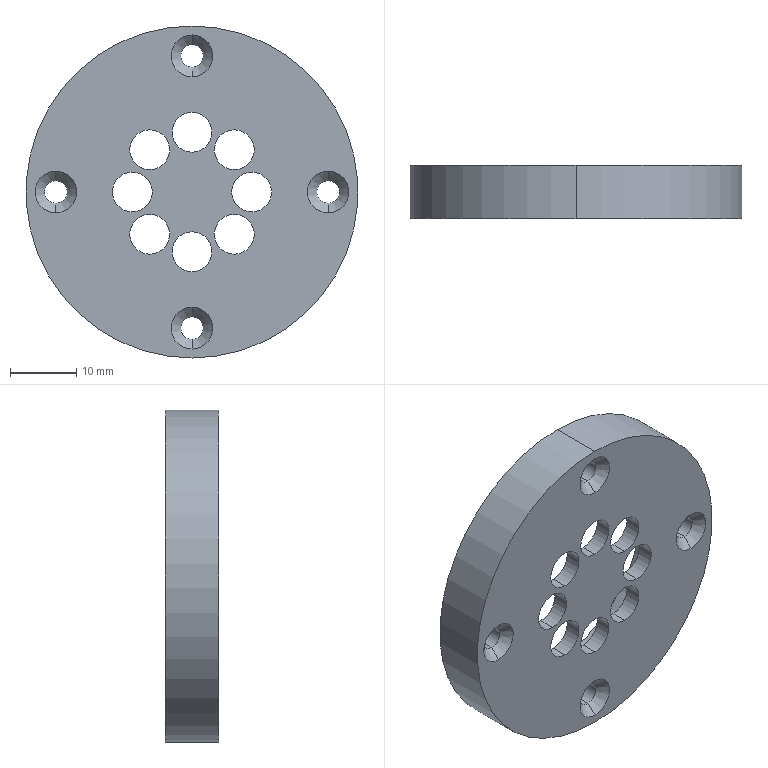Part | SolidWorks | features ICE 2, Extrusion 1, HoleWzd 1 | 1 solid | 39 faces | box 50 x 8 x 50 mm | volume 9503 mm3 | cylinder 28 | cone 8 | plane 3 | commonest cylinder face diameters 6 x16 3.4 x8 35 x2 50 x2
STEP:
#1=CARTESIAN_POINT('',(0.,1.45,-18.8));
#2=VERTEX_POINT('',#1);
#3=CARTESIAN_POINT('',(0.,1.45,-22.2));
#4=VERTEX_POINT('',#3);
#5=CARTESIAN_POINT('',(0.,1.45,-20.5));
#6=DIRECTION('',(0.,-1.,0.));
#7=DIRECTION('',(0.,0.,-1.));
#8=AXIS2_PLACEMENT_3D('',#5,#6,#7);
#9=CIRCLE('',#8,1.7);
#10=EDGE_CURVE('',#2,#4,#9,.T.);
#11=ORIENTED_EDGE('',*,*,#10,.F.);
#12=CARTESIAN_POINT('',(0.,0.,-17.35));
#13=VERTEX_POINT('',#12);
#14=CARTESIAN_POINT('',(0.,0.,-17.35));
#15=DIRECTION('',(0.,-0.7071,0.7071));
#16=VECTOR('',#15,1000.);
#17=LINE('',#14,#16);
#18=EDGE_CURVE('',#2,#13,#17,.T.);
#19=ORIENTED_EDGE('',*,*,#18,.T.);
#20=CARTESIAN_POINT('',(0.,0.,-23.65));
#21=VERTEX_POINT('',#20);
#22=CARTESIAN_POINT('',(0.,0.,-20.5));
#23=DIRECTION('',(0.,-1.,0.));
#24=DIRECTION('',(0.,0.,-1.));
#25=AXIS2_PLACEMENT_3D('',#22,#23,#24);
#26=CIRCLE('',#25,3.15);
#27=EDGE_CURVE('',#13,#21,#26,.T.);
#28=ORIENTED_EDGE('',*,*,#27,.T.);
#29=CARTESIAN_POINT('',(0.,0.,-23.65));
#30=DIRECTION('',(0.,-0.7071,-0.7071));
#31=VECTOR('',#30,1000.);
#32=LINE('',#29,#31);
#33=EDGE_CURVE('',#4,#21,#32,.T.);
#34=ORIENTED_EDGE('',*,*,#33,.F.);
#35=EDGE_LOOP('',(#11,#19,#28,#34));
#36=FACE_OUTER_BOUND('',#35,.T.);
#37=CARTESIAN_POINT('',(0.,0.,-20.5));
#38=DIRECTION('',(0.,-1.,0.));
#39=DIRECTION('',(0.,0.,-1.));
#40=AXIS2_PLACEMENT_3D('',#37,#38,#39);
#41=CONICAL_SURFACE('',#40,3.15,0.7854);
#42=ADVANCED_FACE('',(#36),#41,.F.);
#43=CARTESIAN_POINT('',(0.,8.,-18.8));
#44=VERTEX_POINT('',#43);
#45=CARTESIAN_POINT('',(0.,8.,-22.2));
#46=VERTEX_POINT('',#45);
#47=CARTESIAN_POINT('',(0.,8.,-20.5));
#48=DIRECTION('',(0.,-1.,0.));
#49=DIRECTION('',(0.,0.,-1.));
#50=AXIS2_PLACEMENT_3D('',#47,#48,#49);
#51=CIRCLE('',#50,1.7);
#52=EDGE_CURVE('',#44,#46,#51,.T.);
#53=ORIENTED_EDGE('',*,*,#52,.F.);
#54=CARTESIAN_POINT('',(0.,0.,-18.8));
#55=DIRECTION('',(0.,-1.,0.));
#56=VECTOR('',#55,1000.);
#57=LINE('',#54,#56);
#58=EDGE_CURVE('',#44,#2,#57,.T.);
#59=ORIENTED_EDGE('',*,*,#58,.T.);
#60=ORIENTED_EDGE('',*,*,#10,.T.);
#61=CARTESIAN_POINT('',(0.,0.,-22.2));
#62=DIRECTION('',(0.,-1.,0.));
#63=VECTOR('',#62,1000.);
#64=LINE('',#61,#63);
#65=EDGE_CURVE('',#46,#4,#64,.T.);
#66=ORIENTED_EDGE('',*,*,#65,.F.);
#67=EDGE_LOOP('',(#53,#59,#60,#66));
#68=FACE_OUTER_BOUND('',#67,.T.);
#69=CARTESIAN_POINT('',(0.,0.,-20.5));
#70=DIRECTION('',(0.,-1.,0.));
#71=DIRECTION('',(0.,0.,-1.));
#72=AXIS2_PLACEMENT_3D('',#69,#70,#71);
#73=CYLINDRICAL_SURFACE('',#72,1.7);
#74=ADVANCED_FACE('',(#68),#73,.F.);
#75=CARTESIAN_POINT('',(20.5,1.45,1.7));
#76=VERTEX_POINT('',#75);
#77=CARTESIAN_POINT('',(20.5,1.45,-1.7));
#78=VERTEX_POINT('',#77);
#79=CARTESIAN_POINT('',(20.5,1.45,0.));
#80=DIRECTION('',(0.,-1.,0.));
#81=DIRECTION('',(0.,0.,-1.));
#82=AXIS2_PLACEMENT_3D('',#79,#80,#81);
#83=CIRCLE('',#82,1.7);
#84=EDGE_CURVE('',#76,#78,#83,.T.);
#85=ORIENTED_EDGE('',*,*,#84,.F.);
#86=CARTESIAN_POINT('',(20.5,0.,3.15));
#87=VERTEX_POINT('',#86);
#88=CARTESIAN_POINT('',(20.5,0.,3.15));
#89=DIRECTION('',(0.,-0.7071,0.7071));
#90=VECTOR('',#89,1000.);
#91=LINE('',#88,#90);
#92=EDGE_CURVE('',#76,#87,#91,.T.);
#93=ORIENTED_EDGE('',*,*,#92,.T.);
#94=CARTESIAN_POINT('',(20.5,0.,-3.15));
#95=VERTEX_POINT('',#94);
#96=CARTESIAN_POINT('',(20.5,0.,0.));
#97=DIRECTION('',(0.,-1.,0.));
#98=DIRECTION('',(0.,0.,-1.));
#99=AXIS2_PLACEMENT_3D('',#96,#97,#98);
#100=CIRCLE('',#99,3.15);
#101=EDGE_CURVE('',#87,#95,#100,.T.);
#102=ORIENTED_EDGE('',*,*,#101,.T.);
#103=CARTESIAN_POINT('',(20.5,0.,-3.15));
#104=DIRECTION('',(0.,-0.7071,-0.7071));
#105=VECTOR('',#104,1000.);
#106=LINE('',#103,#105);
#107=EDGE_CURVE('',#78,#95,#106,.T.);
#108=ORIENTED_EDGE('',*,*,#107,.F.);
#109=EDGE_LOOP('',(#85,#93,#102,#108));
#110=FACE_OUTER_BOUND('',#109,.T.);
#111=CARTESIAN_POINT('',(20.5,0.,0.));
#112=DIRECTION('',(0.,-1.,0.));
#113=DIRECTION('',(0.,0.,-1.));
#114=AXIS2_PLACEMENT_3D('',#111,#112,#113);
#115=CONICAL_SURFACE('',#114,3.15,0.7854);
#116=ADVANCED_FACE('',(#110),#115,.F.);
#117=CARTESIAN_POINT('',(20.5,8.,1.7));
#118=VERTEX_POINT('',#117);
#119=CARTESIAN_POINT('',(20.5,8.,-1.7));
#120=VERTEX_POINT('',#119);
#121=CARTESIAN_POINT('',(20.5,8.,0.));
#122=DIRECTION('',(0.,-1.,0.));
#123=DIRECTION('',(0.,0.,-1.));
#124=AXIS2_PLACEMENT_3D('',#121,#122,#123);
#125=CIRCLE('',#124,1.7);
#126=EDGE_CURVE('',#118,#120,#125,.T.);
#127=ORIENTED_EDGE('',*,*,#126,.F.);
#128=CARTESIAN_POINT('',(20.5,0.,1.7));
#129=DIRECTION('',(0.,-1.,0.));
#130=VECTOR('',#129,1000.);
#131=LINE('',#128,#130);
#132=EDGE_CURVE('',#118,#76,#131,.T.);
#133=ORIENTED_EDGE('',*,*,#132,.T.);
#134=ORIENTED_EDGE('',*,*,#84,.T.);
#135=CARTESIAN_POINT('',(20.5,0.,-1.7));
#136=DIRECTION('',(0.,-1.,0.));
#137=VECTOR('',#136,1000.);
#138=LINE('',#135,#137);
#139=EDGE_CURVE('',#120,#78,#138,.T.);
#140=ORIENTED_EDGE('',*,*,#139,.F.);
#141=EDGE_LOOP('',(#127,#133,#134,#140));
#142=FACE_OUTER_BOUND('',#141,.T.);
#143=CARTESIAN_POINT('',(20.5,0.,0.));
#144=DIRECTION('',(0.,-1.,0.));
#145=DIRECTION('',(0.,0.,-1.));
#146=AXIS2_PLACEMENT_3D('',#143,#144,#145);
#147=CYLINDRICAL_SURFACE('',#146,1.7);
#148=ADVANCED_FACE('',(#142),#147,.F.);
#149=CARTESIAN_POINT('',(0.,1.45,22.2));
#150=VERTEX_POINT('',#149);
#151=CARTESIAN_POINT('',(0.,1.45,18.8));
#152=VERTEX_POINT('',#151);
#153=CARTESIAN_POINT('',(0.,1.45,20.5));
#154=DIRECTION('',(0.,-1.,0.));
#155=DIRECTION('',(0.,0.,-1.));
#156=AXIS2_PLACEMENT_3D('',#153,#154,#155);
#157=CIRCLE('',#156,1.7);
#158=EDGE_CURVE('',#150,#152,#157,.T.);
#159=ORIENTED_EDGE('',*,*,#158,.F.);
#160=CARTESIAN_POINT('',(0.,0.,23.65));
#161=VERTEX_POINT('',#160);
#162=CARTESIAN_POINT('',(0.,0.,23.65));
#163=DIRECTION('',(0.,-0.7071,0.7071));
#164=VECTOR('',#163,1000.);
#165=LINE('',#162,#164);
#166=EDGE_CURVE('',#150,#161,#165,.T.);
#167=ORIENTED_EDGE('',*,*,#166,.T.);
#168=CARTESIAN_POINT('',(0.,0.,17.35));
#169=VERTEX_POINT('',#168);
#170=CARTESIAN_POINT('',(0.,0.,20.5));
#171=DIRECTION('',(0.,-1.,0.));
#172=DIRECTION('',(0.,0.,-1.));
#173=AXIS2_PLACEMENT_3D('',#170,#171,#172);
#174=CIRCLE('',#173,3.15);
#175=EDGE_CURVE('',#161,#169,#174,.T.);
#176=ORIENTED_EDGE('',*,*,#175,.T.);
#177=CARTESIAN_POINT('',(0.,0.,17.35));
#178=DIRECTION('',(0.,-0.7071,-0.7071));
#179=VECTOR('',#178,1000.);
#180=LINE('',#177,#179);
#181=EDGE_CURVE('',#152,#169,#180,.T.);
#182=ORIENTED_EDGE('',*,*,#181,.F.);
#183=EDGE_LOOP('',(#159,#167,#176,#182));
#184=FACE_OUTER_BOUND('',#183,.T.);
#185=CARTESIAN_POINT('',(0.,0.,20.5));
#186=DIRECTION('',(0.,-1.,0.));
#187=DIRECTION('',(0.,0.,-1.));
#188=AXIS2_PLACEMENT_3D('',#185,#186,#187);
#189=CONICAL_SURFACE('',#188,3.15,0.7854);
#190=ADVANCED_FACE('',(#184),#189,.F.);
#191=CARTESIAN_POINT('',(0.,8.,22.2));
#192=VERTEX_POINT('',#191);
#193=CARTESIAN_POINT('',(0.,8.,18.8));
#194=VERTEX_POINT('',#193);
#195=CARTESIAN_POINT('',(0.,8.,20.5));
#196=DIRECTION('',(0.,-1.,0.));
#197=DIRECTION('',(0.,0.,-1.));
#198=AXIS2_PLACEMENT_3D('',#195,#196,#197);
#199=CIRCLE('',#198,1.7);
#200=EDGE_CURVE('',#192,#194,#199,.T.);
#201=ORIENTED_EDGE('',*,*,#200,.F.);
#202=CARTESIAN_POINT('',(0.,0.,22.2));
#203=DIRECTION('',(0.,-1.,0.));
#204=VECTOR('',#203,1000.);
#205=LINE('',#202,#204);
#206=EDGE_CURVE('',#192,#150,#205,.T.);
#207=ORIENTED_EDGE('',*,*,#206,.T.);
#208=ORIENTED_EDGE('',*,*,#158,.T.);
#209=CARTESIAN_POINT('',(0.,0.,18.8));
#210=DIRECTION('',(0.,-1.,0.));
#211=VECTOR('',#210,1000.);
#212=LINE('',#209,#211);
#213=EDGE_CURVE('',#194,#152,#212,.T.);
#214=ORIENTED_EDGE('',*,*,#213,.F.);
#215=EDGE_LOOP('',(#201,#207,#208,#214));
#216=FACE_OUTER_BOUND('',#215,.T.);
#217=CARTESIAN_POINT('',(0.,0.,20.5));
#218=DIRECTION('',(0.,-1.,0.));
#219=DIRECTION('',(0.,0.,-1.));
#220=AXIS2_PLACEMENT_3D('',#217,#218,#219);
#221=CYLINDRICAL_SURFACE('',#220,1.7);
#222=ADVANCED_FACE('',(#216),#221,.F.);
#223=CARTESIAN_POINT('',(-20.5,1.45,1.7));
#224=VERTEX_POINT('',#223);
#225=CARTESIAN_POINT('',(-20.5,1.45,-1.7));
#226=VERTEX_POINT('',#225);
#227=CARTESIAN_POINT('',(-20.5,1.45,0.));
#228=DIRECTION('',(0.,-1.,0.));
#229=DIRECTION('',(0.,0.,-1.));
#230=AXIS2_PLACEMENT_3D('',#227,#228,#229);
#231=CIRCLE('',#230,1.7);
#232=EDGE_CURVE('',#224,#226,#231,.T.);
#233=ORIENTED_EDGE('',*,*,#232,.F.);
#234=CARTESIAN_POINT('',(-20.5,0.,3.15));
#235=VERTEX_POINT('',#234);
#236=CARTESIAN_POINT('',(-20.5,0.,3.15));
#237=DIRECTION('',(0.,-0.7071,0.7071));
#238=VECTOR('',#237,1000.);
#239=LINE('',#236,#238);
#240=EDGE_CURVE('',#224,#235,#239,.T.);
#241=ORIENTED_EDGE('',*,*,#240,.T.);
#242=CARTESIAN_POINT('',(-20.5,0.,-3.15));
#243=VERTEX_POINT('',#242);
#244=CARTESIAN_POINT('',(-20.5,0.,0.));
#245=DIRECTION('',(0.,-1.,0.));
#246=DIRECTION('',(0.,0.,-1.));
#247=AXIS2_PLACEMENT_3D('',#244,#245,#246);
#248=CIRCLE('',#247,3.15);
#249=EDGE_CURVE('',#235,#243,#248,.T.);
#250=ORIENTED_EDGE('',*,*,#249,.T.);
#251=CARTESIAN_POINT('',(-20.5,0.,-3.15));
#252=DIRECTION('',(0.,-0.7071,-0.7071));
#253=VECTOR('',#252,1000.);
#254=LINE('',#251,#253);
#255=EDGE_CURVE('',#226,#243,#254,.T.);
#256=ORIENTED_EDGE('',*,*,#255,.F.);
#257=EDGE_LOOP('',(#233,#241,#250,#256));
#258=FACE_OUTER_BOUND('',#257,.T.);
#259=CARTESIAN_POINT('',(-20.5,0.,0.));
#260=DIRECTION('',(0.,-1.,0.));
#261=DIRECTION('',(0.,0.,-1.));
#262=AXIS2_PLACEMENT_3D('',#259,#260,#261);
#263=CONICAL_SURFACE('',#262,3.15,0.7854);
#264=ADVANCED_FACE('',(#258),#263,.F.);
#265=CARTESIAN_POINT('',(-20.5,8.,1.7));
#266=VERTEX_POINT('',#265);
#267=CARTESIAN_POINT('',(-20.5,8.,-1.7));
#268=VERTEX_POINT('',#267);
#269=CARTESIAN_POINT('',(-20.5,8.,0.));
#270=DIRECTION('',(0.,-1.,0.));
#271=DIRECTION('',(0.,0.,-1.));
#272=AXIS2_PLACEMENT_3D('',#269,#270,#271);
#273=CIRCLE('',#272,1.7);
#274=EDGE_CURVE('',#266,#268,#273,.T.);
#275=ORIENTED_EDGE('',*,*,#274,.F.);
#276=CARTESIAN_POINT('',(-20.5,0.,1.7));
#277=DIRECTION('',(0.,-1.,0.));
#278=VECTOR('',#277,1000.);
#279=LINE('',#276,#278);
#280=EDGE_CURVE('',#266,#224,#279,.T.);
#281=ORIENTED_EDGE('',*,*,#280,.T.);
#282=ORIENTED_EDGE('',*,*,#232,.T.);
#283=CARTESIAN_POINT('',(-20.5,0.,-1.7));
#284=DIRECTION('',(0.,-1.,0.));
#285=VECTOR('',#284,1000.);
#286=LINE('',#283,#285);
#287=EDGE_CURVE('',#268,#226,#286,.T.);
#288=ORIENTED_EDGE('',*,*,#287,.F.);
#289=EDGE_LOOP('',(#275,#281,#282,#288));
#290=FACE_OUTER_BOUND('',#289,.T.);
#291=CARTESIAN_POINT('',(-20.5,0.,0.));
#292=DIRECTION('',(0.,-1.,0.));
#293=DIRECTION('',(0.,0.,-1.));
#294=AXIS2_PLACEMENT_3D('',#291,#292,#293);
#295=CYLINDRICAL_SURFACE('',#294,1.7);
#296=ADVANCED_FACE('',(#290),#295,.F.);
#297=CARTESIAN_POINT('',(6.364,2.5,-9.364));
#298=VERTEX_POINT('',#297);
#299=CARTESIAN_POINT('',(6.364,2.5,-3.364));
#300=VERTEX_POINT('',#299);
#301=CARTESIAN_POINT('',(6.364,2.5,-6.364));
#302=DIRECTION('',(0.,1.,0.));
#303=DIRECTION('',(0.,0.,1.));
#304=AXIS2_PLACEMENT_3D('',#301,#302,#303);
#305=CIRCLE('',#304,3.);
#306=EDGE_CURVE('',#298,#300,#305,.T.);
#307=ORIENTED_EDGE('',*,*,#306,.T.);
#308=CARTESIAN_POINT('',(6.364,0.,-3.364));
#309=VERTEX_POINT('',#308);
#310=CARTESIAN_POINT('',(6.364,4.,-3.364));
#311=DIRECTION('',(0.,-1.,0.));
#312=VECTOR('',#311,1000.);
#313=LINE('',#310,#312);
#314=EDGE_CURVE('',#300,#309,#313,.T.);
#315=ORIENTED_EDGE('',*,*,#314,.T.);
#316=CARTESIAN_POINT('',(6.364,0.,-9.364));
#317=VERTEX_POINT('',#316);
#318=CARTESIAN_POINT('',(6.364,0.,-6.364));
#319=DIRECTION('',(0.,-1.,0.));
#320=DIRECTION('',(0.,0.,-1.));
#321=AXIS2_PLACEMENT_3D('',#318,#319,#320);
#322=CIRCLE('',#321,3.);
#323=EDGE_CURVE('',#309,#317,#322,.T.);
#324=ORIENTED_EDGE('',*,*,#323,.T.);
#325=CARTESIAN_POINT('',(6.364,4.,-9.364));
#326=DIRECTION('',(0.,-1.,0.));
#327=VECTOR('',#326,1000.);
#328=LINE('',#325,#327);
#329=EDGE_CURVE('',#298,#317,#328,.T.);
#330=ORIENTED_EDGE('',*,*,#329,.F.);
#331=EDGE_LOOP('',(#307,#315,#324,#330));
#332=FACE_OUTER_BOUND('',#331,.T.);
#333=CARTESIAN_POINT('',(6.364,4.,-6.364));
#334=DIRECTION('',(0.,-1.,0.));
#335=DIRECTION('',(0.,0.,-1.));
#336=AXIS2_PLACEMENT_3D('',#333,#334,#335);
#337=CYLINDRICAL_SURFACE('',#336,3.);
#338=ADVANCED_FACE('',(#332),#337,.F.);
#339=CARTESIAN_POINT('',(9.,2.5,-3.));
#340=VERTEX_POINT('',#339);
#341=CARTESIAN_POINT('',(9.,2.5,3.));
#342=VERTEX_POINT('',#341);
#343=CARTESIAN_POINT('',(9.,2.5,0.));
#344=DIRECTION('',(0.,1.,0.));
#345=DIRECTION('',(0.,0.,1.));
#346=AXIS2_PLACEMENT_3D('',#343,#344,#345);
#347=CIRCLE('',#346,3.);
#348=EDGE_CURVE('',#340,#342,#347,.T.);
#349=ORIENTED_EDGE('',*,*,#348,.T.);
#350=CARTESIAN_POINT('',(9.,0.,3.));
#351=VERTEX_POINT('',#350);
#352=CARTESIAN_POINT('',(9.,4.,3.));
#353=DIRECTION('',(0.,-1.,0.));
#354=VECTOR('',#353,1000.);
#355=LINE('',#352,#354);
#356=EDGE_CURVE('',#342,#351,#355,.T.);
#357=ORIENTED_EDGE('',*,*,#356,.T.);
#358=CARTESIAN_POINT('',(9.,0.,-3.));
#359=VERTEX_POINT('',#358);
#360=CARTESIAN_POINT('',(9.,0.,0.));
#361=DIRECTION('',(0.,-1.,0.));
#362=DIRECTION('',(0.,0.,-1.));
#363=AXIS2_PLACEMENT_3D('',#360,#361,#362);
#364=CIRCLE('',#363,3.);
#365=EDGE_CURVE('',#351,#359,#364,.T.);
#366=ORIENTED_EDGE('',*,*,#365,.T.);
#367=CARTESIAN_POINT('',(9.,4.,-3.));
#368=DIRECTION('',(0.,-1.,0.));
#369=VECTOR('',#368,1000.);
#370=LINE('',#367,#369);
#371=EDGE_CURVE('',#340,#359,#370,.T.);
#372=ORIENTED_EDGE('',*,*,#371,.F.);
#373=EDGE_LOOP('',(#349,#357,#366,#372));
#374=FACE_OUTER_BOUND('',#373,.T.);
#375=CARTESIAN_POINT('',(9.,4.,0.));
#376=DIRECTION('',(0.,-1.,0.));
#377=DIRECTION('',(0.,0.,-1.));
#378=AXIS2_PLACEMENT_3D('',#375,#376,#377);
#379=CYLINDRICAL_SURFACE('',#378,3.);
#380=ADVANCED_FACE('',(#374),#379,.F.);
#381=CARTESIAN_POINT('',(6.364,2.5,3.364));
#382=VERTEX_POINT('',#381);
#383=CARTESIAN_POINT('',(6.364,2.5,9.364));
#384=VERTEX_POINT('',#383);
#385=CARTESIAN_POINT('',(6.364,2.5,6.364));
#386=DIRECTION('',(0.,1.,0.));
#387=DIRECTION('',(0.,0.,1.));
#388=AXIS2_PLACEMENT_3D('',#385,#386,#387);
#389=CIRCLE('',#388,3.);
#390=EDGE_CURVE('',#382,#384,#389,.T.);
#391=ORIENTED_EDGE('',*,*,#390,.T.);
#392=CARTESIAN_POINT('',(6.364,0.,9.364));
#393=VERTEX_POINT('',#392);
#394=CARTESIAN_POINT('',(6.364,4.,9.364));
#395=DIRECTION('',(0.,-1.,0.));
#396=VECTOR('',#395,1000.);
#397=LINE('',#394,#396);
#398=EDGE_CURVE('',#384,#393,#397,.T.);
#399=ORIENTED_EDGE('',*,*,#398,.T.);
#400=CARTESIAN_POINT('',(6.364,0.,3.364));
#401=VERTEX_POINT('',#400);
#402=CARTESIAN_POINT('',(6.364,0.,6.364));
#403=DIRECTION('',(0.,-1.,0.));
#404=DIRECTION('',(0.,0.,-1.));
#405=AXIS2_PLACEMENT_3D('',#402,#403,#404);
#406=CIRCLE('',#405,3.);
#407=EDGE_CURVE('',#393,#401,#406,.T.);
#408=ORIENTED_EDGE('',*,*,#407,.T.);
#409=CARTESIAN_POINT('',(6.364,4.,3.364));
#410=DIRECTION('',(0.,-1.,0.));
#411=VECTOR('',#410,1000.);
#412=LINE('',#409,#411);
#413=EDGE_CURVE('',#382,#401,#412,.T.);
#414=ORIENTED_EDGE('',*,*,#413,.F.);
#415=EDGE_LOOP('',(#391,#399,#408,#414));
#416=FACE_OUTER_BOUND('',#415,.T.);
#417=CARTESIAN_POINT('',(6.364,4.,6.364));
#418=DIRECTION('',(0.,-1.,0.));
#419=DIRECTION('',(0.,0.,-1.));
#420=AXIS2_PLACEMENT_3D('',#417,#418,#419);
#421=CYLINDRICAL_SURFACE('',#420,3.);
#422=ADVANCED_FACE('',(#416),#421,.F.);
#423=CARTESIAN_POINT('',(0.,2.5,6.));
#424=VERTEX_POINT('',#423);
#425=CARTESIAN_POINT('',(0.,2.5,12.));
#426=VERTEX_POINT('',#425);
#427=CARTESIAN_POINT('',(0.,2.5,9.));
#428=DIRECTION('',(0.,1.,0.));
#429=DIRECTION('',(0.,0.,1.));
#430=AXIS2_PLACEMENT_3D('',#427,#428,#429);
#431=CIRCLE('',#430,3.);
#432=EDGE_CURVE('',#424,#426,#431,.T.);
#433=ORIENTED_EDGE('',*,*,#432,.T.);
#434=CARTESIAN_POINT('',(0.,0.,12.));
#435=VERTEX_POINT('',#434);
#436=CARTESIAN_POINT('',(0.,4.,12.));
#437=DIRECTION('',(0.,-1.,0.));
#438=VECTOR('',#437,1000.);
#439=LINE('',#436,#438);
#440=EDGE_CURVE('',#426,#435,#439,.T.);
#441=ORIENTED_EDGE('',*,*,#440,.T.);
#442=CARTESIAN_POINT('',(0.,0.,6.));
#443=VERTEX_POINT('',#442);
#444=CARTESIAN_POINT('',(0.,0.,9.));
#445=DIRECTION('',(0.,-1.,0.));
#446=DIRECTION('',(0.,0.,-1.));
#447=AXIS2_PLACEMENT_3D('',#444,#445,#446);
#448=CIRCLE('',#447,3.);
#449=EDGE_CURVE('',#435,#443,#448,.T.);
#450=ORIENTED_EDGE('',*,*,#449,.T.);
#451=CARTESIAN_POINT('',(0.,4.,6.));
#452=DIRECTION('',(0.,-1.,0.));
#453=VECTOR('',#452,1000.);
#454=LINE('',#451,#453);
#455=EDGE_CURVE('',#424,#443,#454,.T.);
#456=ORIENTED_EDGE('',*,*,#455,.F.);
#457=EDGE_LOOP('',(#433,#441,#450,#456));
#458=FACE_OUTER_BOUND('',#457,.T.);
#459=CARTESIAN_POINT('',(0.,4.,9.));
#460=DIRECTION('',(0.,-1.,0.));
#461=DIRECTION('',(0.,0.,-1.));
#462=AXIS2_PLACEMENT_3D('',#459,#460,#461);
#463=CYLINDRICAL_SURFACE('',#462,3.);
#464=ADVANCED_FACE('',(#458),#463,.F.);
#465=CARTESIAN_POINT('',(-6.364,2.5,3.364));
#466=VERTEX_POINT('',#465);
#467=CARTESIAN_POINT('',(-6.364,2.5,9.364));
#468=VERTEX_POINT('',#467);
#469=CARTESIAN_POINT('',(-6.364,2.5,6.364));
#470=DIRECTION('',(0.,1.,0.));
#471=DIRECTION('',(0.,0.,1.));
#472=AXIS2_PLACEMENT_3D('',#469,#470,#471);
#473=CIRCLE('',#472,3.);
#474=EDGE_CURVE('',#466,#468,#473,.T.);
#475=ORIENTED_EDGE('',*,*,#474,.T.);
#476=CARTESIAN_POINT('',(-6.364,0.,9.364));
#477=VERTEX_POINT('',#476);
#478=CARTESIAN_POINT('',(-6.364,4.,9.364));
#479=DIRECTION('',(0.,-1.,0.));
#480=VECTOR('',#479,1000.);
#481=LINE('',#478,#480);
#482=EDGE_CURVE('',#468,#477,#481,.T.);
#483=ORIENTED_EDGE('',*,*,#482,.T.);
#484=CARTESIAN_POINT('',(-6.364,0.,3.364));
#485=VERTEX_POINT('',#484);
#486=CARTESIAN_POINT('',(-6.364,0.,6.364));
#487=DIRECTION('',(0.,-1.,0.));
#488=DIRECTION('',(0.,0.,-1.));
#489=AXIS2_PLACEMENT_3D('',#486,#487,#488);
#490=CIRCLE('',#489,3.);
#491=EDGE_CURVE('',#477,#485,#490,.T.);
#492=ORIENTED_EDGE('',*,*,#491,.T.);
#493=CARTESIAN_POINT('',(-6.364,4.,3.364));
#494=DIRECTION('',(0.,-1.,0.));
#495=VECTOR('',#494,1000.);
#496=LINE('',#493,#495);
#497=EDGE_CURVE('',#466,#485,#496,.T.);
#498=ORIENTED_EDGE('',*,*,#497,.F.);
#499=EDGE_LOOP('',(#475,#483,#492,#498));
#500=FACE_OUTER_BOUND('',#499,.T.);
#501=CARTESIAN_POINT('',(-6.364,4.,6.364));
#502=DIRECTION('',(0.,-1.,0.));
#503=DIRECTION('',(0.,0.,-1.));
#504=AXIS2_PLACEMENT_3D('',#501,#502,#503);
#505=CYLINDRICAL_SURFACE('',#504,3.);
#506=ADVANCED_FACE('',(#500),#505,.F.);
#507=CARTESIAN_POINT('',(-9.,2.5,-3.));
#508=VERTEX_POINT('',#507);
#509=CARTESIAN_POINT('',(-9.,2.5,3.));
#510=VERTEX_POINT('',#509);
#511=CARTESIAN_POINT('',(-9.,2.5,0.));
#512=DIRECTION('',(0.,1.,0.));
#513=DIRECTION('',(0.,0.,1.));
#514=AXIS2_PLACEMENT_3D('',#511,#512,#513);
#515=CIRCLE('',#514,3.);
#516=EDGE_CURVE('',#508,#510,#515,.T.);
#517=ORIENTED_EDGE('',*,*,#516,.T.);
#518=CARTESIAN_POINT('',(-9.,0.,3.));
#519=VERTEX_POINT('',#518);
#520=CARTESIAN_POINT('',(-9.,4.,3.));
#521=DIRECTION('',(0.,-1.,0.));
#522=VECTOR('',#521,1000.);
#523=LINE('',#520,#522);
#524=EDGE_CURVE('',#510,#519,#523,.T.);
#525=ORIENTED_EDGE('',*,*,#524,.T.);
#526=CARTESIAN_POINT('',(-9.,0.,-3.));
#527=VERTEX_POINT('',#526);
#528=CARTESIAN_POINT('',(-9.,0.,0.));
#529=DIRECTION('',(0.,-1.,0.));
#530=DIRECTION('',(0.,0.,-1.));
#531=AXIS2_PLACEMENT_3D('',#528,#529,#530);
#532=CIRCLE('',#531,3.);
#533=EDGE_CURVE('',#519,#527,#532,.T.);
#534=ORIENTED_EDGE('',*,*,#533,.T.);
#535=CARTESIAN_POINT('',(-9.,4.,-3.));
#536=DIRECTION('',(0.,-1.,0.));
#537=VECTOR('',#536,1000.);
#538=LINE('',#535,#537);
#539=EDGE_CURVE('',#508,#527,#538,.T.);
#540=ORIENTED_EDGE('',*,*,#539,.F.);
#541=EDGE_LOOP('',(#517,#525,#534,#540));
#542=FACE_OUTER_BOUND('',#541,.T.);
#543=CARTESIAN_POINT('',(-9.,4.,0.));
#544=DIRECTION('',(0.,-1.,0.));
#545=DIRECTION('',(0.,0.,-1.));
#546=AXIS2_PLACEMENT_3D('',#543,#544,#545);
#547=CYLINDRICAL_SURFACE('',#546,3.);
#548=ADVANCED_FACE('',(#542),#547,.F.);
#549=CARTESIAN_POINT('',(-6.364,2.5,-9.364));
#550=VERTEX_POINT('',#549);
#551=CARTESIAN_POINT('',(-6.364,2.5,-3.364));
#552=VERTEX_POINT('',#551);
#553=CARTESIAN_POINT('',(-6.364,2.5,-6.364));
#554=DIRECTION('',(0.,1.,0.));
#555=DIRECTION('',(0.,0.,1.));
#556=AXIS2_PLACEMENT_3D('',#553,#554,#555);
#557=CIRCLE('',#556,3.);
#558=EDGE_CURVE('',#550,#552,#557,.T.);
#559=ORIENTED_EDGE('',*,*,#558,.T.);
#560=CARTESIAN_POINT('',(-6.364,0.,-3.364));
#561=VERTEX_POINT('',#560);
#562=CARTESIAN_POINT('',(-6.364,4.,-3.364));
#563=DIRECTION('',(0.,-1.,0.));
#564=VECTOR('',#563,1000.);
#565=LINE('',#562,#564);
#566=EDGE_CURVE('',#552,#561,#565,.T.);
#567=ORIENTED_EDGE('',*,*,#566,.T.);
#568=CARTESIAN_POINT('',(-6.364,0.,-9.364));
#569=VERTEX_POINT('',#568);
#570=CARTESIAN_POINT('',(-6.364,0.,-6.364));
#571=DIRECTION('',(0.,-1.,0.));
#572=DIRECTION('',(0.,0.,-1.));
#573=AXIS2_PLACEMENT_3D('',#570,#571,#572);
#574=CIRCLE('',#573,3.);
#575=EDGE_CURVE('',#561,#569,#574,.T.);
#576=ORIENTED_EDGE('',*,*,#575,.T.);
#577=CARTESIAN_POINT('',(-6.364,4.,-9.364));
#578=DIRECTION('',(0.,-1.,0.));
#579=VECTOR('',#578,1000.);
#580=LINE('',#577,#579);
#581=EDGE_CURVE('',#550,#569,#580,.T.);
#582=ORIENTED_EDGE('',*,*,#581,.F.);
#583=EDGE_LOOP('',(#559,#567,#576,#582));
#584=FACE_OUTER_BOUND('',#583,.T.);
#585=CARTESIAN_POINT('',(-6.364,4.,-6.364));
#586=DIRECTION('',(0.,-1.,0.));
#587=DIRECTION('',(0.,0.,-1.));
#588=AXIS2_PLACEMENT_3D('',#585,#586,#587);
#589=CYLINDRICAL_SURFACE('',#588,3.);
#590=ADVANCED_FACE('',(#584),#589,.F.);
#591=CARTESIAN_POINT('',(0.,2.5,-12.));
#592=VERTEX_POINT('',#591);
#593=CARTESIAN_POINT('',(0.,2.5,-6.));
#594=VERTEX_POINT('',#593);
#595=CARTESIAN_POINT('',(0.,2.5,-9.));
#596=DIRECTION('',(0.,1.,0.));
#597=DIRECTION('',(0.,0.,1.));
#598=AXIS2_PLACEMENT_3D('',#595,#596,#597);
#599=CIRCLE('',#598,3.);
#600=EDGE_CURVE('',#592,#594,#599,.T.);
#601=ORIENTED_EDGE('',*,*,#600,.T.);
#602=CARTESIAN_POINT('',(0.,0.,-6.));
#603=VERTEX_POINT('',#602);
#604=CARTESIAN_POINT('',(0.,4.,-6.));
#605=DIRECTION('',(0.,-1.,0.));
#606=VECTOR('',#605,1000.);
#607=LINE('',#604,#606);
#608=EDGE_CURVE('',#594,#603,#607,.T.);
#609=ORIENTED_EDGE('',*,*,#608,.T.);
#610=CARTESIAN_POINT('',(0.,0.,-12.));
#611=VERTEX_POINT('',#610);
#612=CARTESIAN_POINT('',(0.,0.,-9.));
#613=DIRECTION('',(0.,-1.,0.));
#614=DIRECTION('',(0.,0.,-1.));
#615=AXIS2_PLACEMENT_3D('',#612,#613,#614);
#616=CIRCLE('',#615,3.);
#617=EDGE_CURVE('',#603,#611,#616,.T.);
#618=ORIENTED_EDGE('',*,*,#617,.T.);
#619=CARTESIAN_POINT('',(0.,4.,-12.));
#620=DIRECTION('',(0.,-1.,0.));
#621=VECTOR('',#620,1000.);
#622=LINE('',#619,#621);
#623=EDGE_CURVE('',#592,#611,#622,.T.);
#624=ORIENTED_EDGE('',*,*,#623,.F.);
#625=EDGE_LOOP('',(#601,#609,#618,#624));
#626=FACE_OUTER_BOUND('',#625,.T.);
#627=CARTESIAN_POINT('',(0.,4.,-9.));
#628=DIRECTION('',(0.,-1.,0.));
#629=DIRECTION('',(0.,0.,-1.));
#630=AXIS2_PLACEMENT_3D('',#627,#628,#629);
#631=CYLINDRICAL_SURFACE('',#630,3.);
#632=ADVANCED_FACE('',(#626),#631,.F.);
#633=CARTESIAN_POINT('',(0.,2.5,-17.5));
#634=VERTEX_POINT('',#633);
#635=CARTESIAN_POINT('',(0.,2.5,17.5));
#636=VERTEX_POINT('',#635);
#637=CARTESIAN_POINT('',(0.,2.5,0.));
#638=DIRECTION('',(0.,1.,0.));
#639=DIRECTION('',(0.,0.,1.));
#640=AXIS2_PLACEMENT_3D('',#637,#638,#639);
#641=CIRCLE('',#640,17.5);
#642=EDGE_CURVE('',#634,#636,#641,.T.);
#643=ORIENTED_EDGE('',*,*,#642,.F.);
#644=CARTESIAN_POINT('',(0.,8.,-17.5));
#645=VERTEX_POINT('',#644);
#646=CARTESIAN_POINT('',(0.,2.5,-17.5));
#647=DIRECTION('',(0.,1.,0.));
#648=VECTOR('',#647,1000.);
#649=LINE('',#646,#648);
#650=EDGE_CURVE('',#634,#645,#649,.T.);
#651=ORIENTED_EDGE('',*,*,#650,.T.);
#652=CARTESIAN_POINT('',(0.,8.,17.5));
#653=VERTEX_POINT('',#652);
#654=CARTESIAN_POINT('',(0.,8.,0.));
#655=DIRECTION('',(0.,1.,0.));
#656=DIRECTION('',(0.,0.,1.));
#657=AXIS2_PLACEMENT_3D('',#654,#655,#656);
#658=CIRCLE('',#657,17.5);
#659=EDGE_CURVE('',#645,#653,#658,.T.);
#660=ORIENTED_EDGE('',*,*,#659,.T.);
#661=CARTESIAN_POINT('',(0.,2.5,17.5));
#662=DIRECTION('',(0.,1.,0.));
#663=VECTOR('',#662,1000.);
#664=LINE('',#661,#663);
#665=EDGE_CURVE('',#636,#653,#664,.T.);
#666=ORIENTED_EDGE('',*,*,#665,.F.);
#667=EDGE_LOOP('',(#643,#651,#660,#666));
#668=FACE_OUTER_BOUND('',#667,.T.);
#669=CARTESIAN_POINT('',(0.,2.5,0.));
#670=DIRECTION('',(0.,1.,0.));
#671=DIRECTION('',(0.,0.,1.));
#672=AXIS2_PLACEMENT_3D('',#669,#670,#671);
#673=CYLINDRICAL_SURFACE('',#672,17.5);
#674=ADVANCED_FACE('',(#668),#673,.F.);
#675=CARTESIAN_POINT('',(0.,8.,25.));
#676=VERTEX_POINT('',#675);
#677=CARTESIAN_POINT('',(0.,8.,-25.));
#678=VERTEX_POINT('',#677);
#679=CARTESIAN_POINT('',(0.,8.,0.));
#680=DIRECTION('',(0.,1.,0.));
#681=DIRECTION('',(0.,0.,1.));
#682=AXIS2_PLACEMENT_3D('',#679,#680,#681);
#683=CIRCLE('',#682,25.);
#684=EDGE_CURVE('',#676,#678,#683,.T.);
#685=ORIENTED_EDGE('',*,*,#684,.F.);
#686=CARTESIAN_POINT('',(0.,0.,25.));
#687=VERTEX_POINT('',#686);
#688=CARTESIAN_POINT('',(0.,8.,25.));
#689=DIRECTION('',(0.,-1.,0.));
#690=VECTOR('',#689,1000.);
#691=LINE('',#688,#690);
#692=EDGE_CURVE('',#676,#687,#691,.T.);
#693=ORIENTED_EDGE('',*,*,#692,.T.);
#694=CARTESIAN_POINT('',(0.,0.,-25.));
#695=VERTEX_POINT('',#694);
#696=CARTESIAN_POINT('',(0.,0.,0.));
#697=DIRECTION('',(0.,1.,0.));
#698=DIRECTION('',(0.,0.,1.));
#699=AXIS2_PLACEMENT_3D('',#696,#697,#698);
#700=CIRCLE('',#699,25.);
#701=EDGE_CURVE('',#687,#695,#700,.T.);
#702=ORIENTED_EDGE('',*,*,#701,.T.);
#703=CARTESIAN_POINT('',(0.,8.,-25.));
#704=DIRECTION('',(0.,-1.,0.));
#705=VECTOR('',#704,1000.);
#706=LINE('',#703,#705);
#707=EDGE_CURVE('',#678,#695,#706,.T.);
#708=ORIENTED_EDGE('',*,*,#707,.F.);
#709=EDGE_LOOP('',(#685,#693,#702,#708));
#710=FACE_OUTER_BOUND('',#709,.T.);
#711=CARTESIAN_POINT('',(0.,8.,0.));
#712=DIRECTION('',(0.,-1.,0.));
#713=DIRECTION('',(0.,0.,-1.));
#714=AXIS2_PLACEMENT_3D('',#711,#712,#713);
#715=CYLINDRICAL_SURFACE('',#714,25.);
#716=ADVANCED_FACE('',(#710),#715,.T.);
#717=CARTESIAN_POINT('',(20.5,8.,0.));
#718=DIRECTION('',(0.,-1.,0.));
#719=DIRECTION('',(0.,0.,-1.));
#720=AXIS2_PLACEMENT_3D('',#717,#718,#719);
#721=CIRCLE('',#720,1.7);
#722=EDGE_CURVE('',#120,#118,#721,.T.);
#723=ORIENTED_EDGE('',*,*,#722,.T.);
#724=ORIENTED_EDGE('',*,*,#126,.T.);
#725=EDGE_LOOP('',(#723,#724));
#726=FACE_BOUND('',#725,.T.);
#727=CARTESIAN_POINT('',(-20.5,8.,0.));
#728=DIRECTION('',(0.,-1.,0.));
#729=DIRECTION('',(0.,0.,-1.));
#730=AXIS2_PLACEMENT_3D('',#727,#728,#729);
#731=CIRCLE('',#730,1.7);
#732=EDGE_CURVE('',#268,#266,#731,.T.);
#733=ORIENTED_EDGE('',*,*,#732,.T.);
#734=ORIENTED_EDGE('',*,*,#274,.T.);
#735=EDGE_LOOP('',(#733,#734));
#736=FACE_BOUND('',#735,.T.);
#737=CARTESIAN_POINT('',(0.,8.,0.));
#738=DIRECTION('',(0.,1.,0.));
#739=DIRECTION('',(0.,0.,1.));
#740=AXIS2_PLACEMENT_3D('',#737,#738,#739);
#741=CIRCLE('',#740,17.5);
#742=EDGE_CURVE('',#653,#645,#741,.T.);
#743=ORIENTED_EDGE('',*,*,#742,.F.);
#744=ORIENTED_EDGE('',*,*,#659,.F.);
#745=EDGE_LOOP('',(#743,#744));
#746=FACE_BOUND('',#745,.T.);
#747=CARTESIAN_POINT('',(0.,8.,0.));
#748=DIRECTION('',(0.,1.,0.));
#749=DIRECTION('',(0.,0.,1.));
#750=AXIS2_PLACEMENT_3D('',#747,#748,#749);
#751=CIRCLE('',#750,25.);
#752=EDGE_CURVE('',#678,#676,#751,.T.);
#753=ORIENTED_EDGE('',*,*,#752,.T.);
#754=ORIENTED_EDGE('',*,*,#684,.T.);
#755=EDGE_LOOP('',(#753,#754));
#756=FACE_OUTER_BOUND('',#755,.T.);
#757=CARTESIAN_POINT('',(0.,8.,20.5));
#758=DIRECTION('',(0.,-1.,0.));
#759=DIRECTION('',(0.,0.,-1.));
#760=AXIS2_PLACEMENT_3D('',#757,#758,#759);
#761=CIRCLE('',#760,1.7);
#762=EDGE_CURVE('',#194,#192,#761,.T.);
#763=ORIENTED_EDGE('',*,*,#762,.T.);
#764=ORIENTED_EDGE('',*,*,#200,.T.);
#765=EDGE_LOOP('',(#763,#764));
#766=FACE_BOUND('',#765,.T.);
#767=CARTESIAN_POINT('',(0.,8.,-20.5));
#768=DIRECTION('',(0.,-1.,0.));
#769=DIRECTION('',(0.,0.,-1.));
#770=AXIS2_PLACEMENT_3D('',#767,#768,#769);
#771=CIRCLE('',#770,1.7);
#772=EDGE_CURVE('',#46,#44,#771,.T.);
#773=ORIENTED_EDGE('',*,*,#772,.T.);
#774=ORIENTED_EDGE('',*,*,#52,.T.);
#775=EDGE_LOOP('',(#773,#774));
#776=FACE_BOUND('',#775,.T.);
#777=CARTESIAN_POINT('',(0.,8.,0.));
#778=DIRECTION('',(0.,1.,0.));
#779=DIRECTION('',(0.,0.,1.));
#780=AXIS2_PLACEMENT_3D('',#777,#778,#779);
#781=PLANE('',#780);
#782=ADVANCED_FACE('',(#726,#736,#746,#756,#766,#776),#781,.T.);
#783=CARTESIAN_POINT('',(20.5,0.,0.));
#784=DIRECTION('',(0.,-1.,0.));
#785=DIRECTION('',(0.,0.,-1.));
#786=AXIS2_PLACEMENT_3D('',#783,#784,#785);
#787=CIRCLE('',#786,3.15);
#788=EDGE_CURVE('',#95,#87,#787,.T.);
#789=ORIENTED_EDGE('',*,*,#788,.F.);
#790=ORIENTED_EDGE('',*,*,#101,.F.);
#791=EDGE_LOOP('',(#789,#790));
#792=FACE_BOUND('',#791,.T.);
#793=CARTESIAN_POINT('',(-20.5,0.,0.));
#794=DIRECTION('',(0.,-1.,0.));
#795=DIRECTION('',(0.,0.,-1.));
#796=AXIS2_PLACEMENT_3D('',#793,#794,#795);
#797=CIRCLE('',#796,3.15);
#798=EDGE_CURVE('',#243,#235,#797,.T.);
#799=ORIENTED_EDGE('',*,*,#798,.F.);
#800=ORIENTED_EDGE('',*,*,#249,.F.);
#801=EDGE_LOOP('',(#799,#800));
#802=FACE_BOUND('',#801,.T.);
#803=CARTESIAN_POINT('',(6.364,0.,-6.364));
#804=DIRECTION('',(0.,-1.,0.));
#805=DIRECTION('',(0.,0.,-1.));
#806=AXIS2_PLACEMENT_3D('',#803,#804,#805);
#807=CIRCLE('',#806,3.);
#808=EDGE_CURVE('',#317,#309,#807,.T.);
#809=ORIENTED_EDGE('',*,*,#808,.F.);
#810=ORIENTED_EDGE('',*,*,#323,.F.);
#811=EDGE_LOOP('',(#809,#810));
#812=FACE_BOUND('',#811,.T.);
#813=CARTESIAN_POINT('',(9.,0.,0.));
#814=DIRECTION('',(0.,-1.,0.));
#815=DIRECTION('',(0.,0.,-1.));
#816=AXIS2_PLACEMENT_3D('',#813,#814,#815);
#817=CIRCLE('',#816,3.);
#818=EDGE_CURVE('',#359,#351,#817,.T.);
#819=ORIENTED_EDGE('',*,*,#818,.F.);
#820=ORIENTED_EDGE('',*,*,#365,.F.);
#821=EDGE_LOOP('',(#819,#820));
#822=FACE_BOUND('',#821,.T.);
#823=CARTESIAN_POINT('',(6.364,0.,6.364));
#824=DIRECTION('',(0.,-1.,0.));
#825=DIRECTION('',(0.,0.,-1.));
#826=AXIS2_PLACEMENT_3D('',#823,#824,#825);
#827=CIRCLE('',#826,3.);
#828=EDGE_CURVE('',#401,#393,#827,.T.);
#829=ORIENTED_EDGE('',*,*,#828,.F.);
#830=ORIENTED_EDGE('',*,*,#407,.F.);
#831=EDGE_LOOP('',(#829,#830));
#832=FACE_BOUND('',#831,.T.);
#833=CARTESIAN_POINT('',(0.,0.,9.));
#834=DIRECTION('',(0.,-1.,0.));
#835=DIRECTION('',(0.,0.,-1.));
#836=AXIS2_PLACEMENT_3D('',#833,#834,#835);
#837=CIRCLE('',#836,3.);
#838=EDGE_CURVE('',#443,#435,#837,.T.);
#839=ORIENTED_EDGE('',*,*,#838,.F.);
#840=ORIENTED_EDGE('',*,*,#449,.F.);
#841=EDGE_LOOP('',(#839,#840));
#842=FACE_BOUND('',#841,.T.);
#843=CARTESIAN_POINT('',(-6.364,0.,6.364));
#844=DIRECTION('',(0.,-1.,0.));
#845=DIRECTION('',(0.,0.,-1.));
#846=AXIS2_PLACEMENT_3D('',#843,#844,#845);
#847=CIRCLE('',#846,3.);
#848=EDGE_CURVE('',#485,#477,#847,.T.);
#849=ORIENTED_EDGE('',*,*,#848,.F.);
#850=ORIENTED_EDGE('',*,*,#491,.F.);
#851=EDGE_LOOP('',(#849,#850));
#852=FACE_BOUND('',#851,.T.);
#853=CARTESIAN_POINT('',(-9.,0.,0.));
#854=DIRECTION('',(0.,-1.,0.));
#855=DIRECTION('',(0.,0.,-1.));
#856=AXIS2_PLACEMENT_3D('',#853,#854,#855);
#857=CIRCLE('',#856,3.);
#858=EDGE_CURVE('',#527,#519,#857,.T.);
#859=ORIENTED_EDGE('',*,*,#858,.F.);
#860=ORIENTED_EDGE('',*,*,#533,.F.);
#861=EDGE_LOOP('',(#859,#860));
#862=FACE_BOUND('',#861,.T.);
#863=CARTESIAN_POINT('',(-6.364,0.,-6.364));
#864=DIRECTION('',(0.,-1.,0.));
#865=DIRECTION('',(0.,0.,-1.));
#866=AXIS2_PLACEMENT_3D('',#863,#864,#865);
#867=CIRCLE('',#866,3.);
#868=EDGE_CURVE('',#569,#561,#867,.T.);
#869=ORIENTED_EDGE('',*,*,#868,.F.);
#870=ORIENTED_EDGE('',*,*,#575,.F.);
#871=EDGE_LOOP('',(#869,#870));
#872=FACE_BOUND('',#871,.T.);
#873=CARTESIAN_POINT('',(0.,0.,-9.));
#874=DIRECTION('',(0.,-1.,0.));
#875=DIRECTION('',(0.,0.,-1.));
#876=AXIS2_PLACEMENT_3D('',#873,#874,#875);
#877=CIRCLE('',#876,3.);
#878=EDGE_CURVE('',#611,#603,#877,.T.);
#879=ORIENTED_EDGE('',*,*,#878,.F.);
#880=ORIENTED_EDGE('',*,*,#617,.F.);
#881=EDGE_LOOP('',(#879,#880));
#882=FACE_BOUND('',#881,.T.);
#883=CARTESIAN_POINT('',(0.,0.,0.));
#884=DIRECTION('',(0.,1.,0.));
#885=DIRECTION('',(0.,0.,1.));
#886=AXIS2_PLACEMENT_3D('',#883,#884,#885);
#887=CIRCLE('',#886,25.);
#888=EDGE_CURVE('',#695,#687,#887,.T.);
#889=ORIENTED_EDGE('',*,*,#888,.F.);
#890=ORIENTED_EDGE('',*,*,#701,.F.);
#891=EDGE_LOOP('',(#889,#890));
#892=FACE_OUTER_BOUND('',#891,.T.);
#893=CARTESIAN_POINT('',(0.,0.,20.5));
#894=DIRECTION('',(0.,-1.,0.));
#895=DIRECTION('',(0.,0.,-1.));
#896=AXIS2_PLACEMENT_3D('',#893,#894,#895);
#897=CIRCLE('',#896,3.15);
#898=EDGE_CURVE('',#169,#161,#897,.T.);
#899=ORIENTED_EDGE('',*,*,#898,.F.);
#900=ORIENTED_EDGE('',*,*,#175,.F.);
#901=EDGE_LOOP('',(#899,#900));
#902=FACE_BOUND('',#901,.T.);
#903=CARTESIAN_POINT('',(0.,0.,-20.5));
#904=DIRECTION('',(0.,-1.,0.));
#905=DIRECTION('',(0.,0.,-1.));
#906=AXIS2_PLACEMENT_3D('',#903,#904,#905);
#907=CIRCLE('',#906,3.15);
#908=EDGE_CURVE('',#21,#13,#907,.T.);
#909=ORIENTED_EDGE('',*,*,#908,.F.);
#910=ORIENTED_EDGE('',*,*,#27,.F.);
#911=EDGE_LOOP('',(#909,#910));
#912=FACE_BOUND('',#911,.T.);
#913=CARTESIAN_POINT('',(0.,0.,0.));
#914=DIRECTION('',(0.,1.,0.));
#915=DIRECTION('',(0.,0.,1.));
#916=AXIS2_PLACEMENT_3D('',#913,#914,#915);
#917=PLANE('',#916);
#918=ADVANCED_FACE('',(#792,#802,#812,#822,#832,#842,#852,#862,#872,#882,#892,#902,#912),#917,.F.);
#919=ORIENTED_EDGE('',*,*,#692,.F.);
#920=ORIENTED_EDGE('',*,*,#752,.F.);
#921=ORIENTED_EDGE('',*,*,#707,.T.);
#922=ORIENTED_EDGE('',*,*,#888,.T.);
#923=EDGE_LOOP('',(#919,#920,#921,#922));
#924=FACE_OUTER_BOUND('',#923,.T.);
#925=CARTESIAN_POINT('',(0.,8.,0.));
#926=DIRECTION('',(0.,-1.,0.));
#927=DIRECTION('',(0.,0.,-1.));
#928=AXIS2_PLACEMENT_3D('',#925,#926,#927);
#929=CYLINDRICAL_SURFACE('',#928,25.);
#930=ADVANCED_FACE('',(#924),#929,.T.);
#931=ORIENTED_EDGE('',*,*,#650,.F.);
#932=CARTESIAN_POINT('',(0.,2.5,0.));
#933=DIRECTION('',(0.,1.,0.));
#934=DIRECTION('',(0.,0.,1.));
#935=AXIS2_PLACEMENT_3D('',#932,#933,#934);
#936=CIRCLE('',#935,17.5);
#937=EDGE_CURVE('',#636,#634,#936,.T.);
#938=ORIENTED_EDGE('',*,*,#937,.F.);
#939=ORIENTED_EDGE('',*,*,#665,.T.);
#940=ORIENTED_EDGE('',*,*,#742,.T.);
#941=EDGE_LOOP('',(#931,#938,#939,#940));
#942=FACE_OUTER_BOUND('',#941,.T.);
#943=CARTESIAN_POINT('',(0.,2.5,0.));
#944=DIRECTION('',(0.,1.,0.));
#945=DIRECTION('',(0.,0.,1.));
#946=AXIS2_PLACEMENT_3D('',#943,#944,#945);
#947=CYLINDRICAL_SURFACE('',#946,17.5);
#948=ADVANCED_FACE('',(#942),#947,.F.);
#949=ORIENTED_EDGE('',*,*,#306,.F.);
#950=CARTESIAN_POINT('',(6.364,2.5,-6.364));
#951=DIRECTION('',(0.,1.,0.));
#952=DIRECTION('',(0.,0.,1.));
#953=AXIS2_PLACEMENT_3D('',#950,#951,#952);
#954=CIRCLE('',#953,3.);
#955=EDGE_CURVE('',#300,#298,#954,.T.);
#956=ORIENTED_EDGE('',*,*,#955,.F.);
#957=EDGE_LOOP('',(#949,#956));
#958=FACE_BOUND('',#957,.T.);
#959=ORIENTED_EDGE('',*,*,#348,.F.);
#960=CARTESIAN_POINT('',(9.,2.5,0.));
#961=DIRECTION('',(0.,1.,0.));
#962=DIRECTION('',(0.,0.,1.));
#963=AXIS2_PLACEMENT_3D('',#960,#961,#962);
#964=CIRCLE('',#963,3.);
#965=EDGE_CURVE('',#342,#340,#964,.T.);
#966=ORIENTED_EDGE('',*,*,#965,.F.);
#967=EDGE_LOOP('',(#959,#966));
#968=FACE_BOUND('',#967,.T.);
#969=ORIENTED_EDGE('',*,*,#390,.F.);
#970=CARTESIAN_POINT('',(6.364,2.5,6.364));
#971=DIRECTION('',(0.,1.,0.));
#972=DIRECTION('',(0.,0.,1.));
#973=AXIS2_PLACEMENT_3D('',#970,#971,#972);
#974=CIRCLE('',#973,3.);
#975=EDGE_CURVE('',#384,#382,#974,.T.);
#976=ORIENTED_EDGE('',*,*,#975,.F.);
#977=EDGE_LOOP('',(#969,#976));
#978=FACE_BOUND('',#977,.T.);
#979=ORIENTED_EDGE('',*,*,#432,.F.);
#980=CARTESIAN_POINT('',(0.,2.5,9.));
#981=DIRECTION('',(0.,1.,0.));
#982=DIRECTION('',(0.,0.,1.));
#983=AXIS2_PLACEMENT_3D('',#980,#981,#982);
#984=CIRCLE('',#983,3.);
#985=EDGE_CURVE('',#426,#424,#984,.T.);
#986=ORIENTED_EDGE('',*,*,#985,.F.);
#987=EDGE_LOOP('',(#979,#986));
#988=FACE_BOUND('',#987,.T.);
#989=ORIENTED_EDGE('',*,*,#474,.F.);
#990=CARTESIAN_POINT('',(-6.364,2.5,6.364));
#991=DIRECTION('',(0.,1.,0.));
#992=DIRECTION('',(0.,0.,1.));
#993=AXIS2_PLACEMENT_3D('',#990,#991,#992);
#994=CIRCLE('',#993,3.);
#995=EDGE_CURVE('',#468,#466,#994,.T.);
#996=ORIENTED_EDGE('',*,*,#995,.F.);
#997=EDGE_LOOP('',(#989,#996));
#998=FACE_BOUND('',#997,.T.);
#999=ORIENTED_EDGE('',*,*,#516,.F.);
#1000=CARTESIAN_POINT('',(-9.,2.5,0.));
#1001=DIRECTION('',(0.,1.,0.));
#1002=DIRECTION('',(0.,0.,1.));
#1003=AXIS2_PLACEMENT_3D('',#1000,#1001,#1002);
#1004=CIRCLE('',#1003,3.);
#1005=EDGE_CURVE('',#510,#508,#1004,.T.);
#1006=ORIENTED_EDGE('',*,*,#1005,.F.);
#1007=EDGE_LOOP('',(#999,#1006));
#1008=FACE_BOUND('',#1007,.T.);
#1009=ORIENTED_EDGE('',*,*,#558,.F.);
#1010=CARTESIAN_POINT('',(-6.364,2.5,-6.364));
#1011=DIRECTION('',(0.,1.,0.));
#1012=DIRECTION('',(0.,0.,1.));
#1013=AXIS2_PLACEMENT_3D('',#1010,#1011,#1012);
#1014=CIRCLE('',#1013,3.);
#1015=EDGE_CURVE('',#552,#550,#1014,.T.);
#1016=ORIENTED_EDGE('',*,*,#1015,.F.);
#1017=EDGE_LOOP('',(#1009,#1016));
#1018=FACE_BOUND('',#1017,.T.);
#1019=ORIENTED_EDGE('',*,*,#600,.F.);
#1020=CARTESIAN_POINT('',(0.,2.5,-9.));
#1021=DIRECTION('',(0.,1.,0.));
#1022=DIRECTION('',(0.,0.,1.));
#1023=AXIS2_PLACEMENT_3D('',#1020,#1021,#1022);
#1024=CIRCLE('',#1023,3.);
#1025=EDGE_CURVE('',#594,#592,#1024,.T.);
#1026=ORIENTED_EDGE('',*,*,#1025,.F.);
#1027=EDGE_LOOP('',(#1019,#1026));
#1028=FACE_BOUND('',#1027,.T.);
#1029=ORIENTED_EDGE('',*,*,#937,.T.);
#1030=ORIENTED_EDGE('',*,*,#642,.T.);
#1031=EDGE_LOOP('',(#1029,#1030));
#1032=FACE_OUTER_BOUND('',#1031,.T.);
#1033=CARTESIAN_POINT('',(0.,2.5,0.));
#1034=DIRECTION('',(0.,1.,0.));
#1035=DIRECTION('',(0.,0.,1.));
#1036=AXIS2_PLACEMENT_3D('',#1033,#1034,#1035);
#1037=PLANE('',#1036);
#1038=ADVANCED_FACE('',(#958,#968,#978,#988,#998,#1008,#1018,#1028,#1032),#1037,.T.);
#1039=ORIENTED_EDGE('',*,*,#608,.F.);
#1040=ORIENTED_EDGE('',*,*,#1025,.T.);
#1041=ORIENTED_EDGE('',*,*,#623,.T.);
#1042=ORIENTED_EDGE('',*,*,#878,.T.);
#1043=EDGE_LOOP('',(#1039,#1040,#1041,#1042));
#1044=FACE_OUTER_BOUND('',#1043,.T.);
#1045=CARTESIAN_POINT('',(0.,4.,-9.));
#1046=DIRECTION('',(0.,-1.,0.));
#1047=DIRECTION('',(0.,0.,-1.));
#1048=AXIS2_PLACEMENT_3D('',#1045,#1046,#1047);
#1049=CYLINDRICAL_SURFACE('',#1048,3.);
#1050=ADVANCED_FACE('',(#1044),#1049,.F.);
#1051=ORIENTED_EDGE('',*,*,#566,.F.);
#1052=ORIENTED_EDGE('',*,*,#1015,.T.);
#1053=ORIENTED_EDGE('',*,*,#581,.T.);
#1054=ORIENTED_EDGE('',*,*,#868,.T.);
#1055=EDGE_LOOP('',(#1051,#1052,#1053,#1054));
#1056=FACE_OUTER_BOUND('',#1055,.T.);
#1057=CARTESIAN_POINT('',(-6.364,4.,-6.364));
#1058=DIRECTION('',(0.,-1.,0.));
#1059=DIRECTION('',(0.,0.,-1.));
#1060=AXIS2_PLACEMENT_3D('',#1057,#1058,#1059);
#1061=CYLINDRICAL_SURFACE('',#1060,3.);
#1062=ADVANCED_FACE('',(#1056),#1061,.F.);
#1063=ORIENTED_EDGE('',*,*,#524,.F.);
#1064=ORIENTED_EDGE('',*,*,#1005,.T.);
#1065=ORIENTED_EDGE('',*,*,#539,.T.);
#1066=ORIENTED_EDGE('',*,*,#858,.T.);
#1067=EDGE_LOOP('',(#1063,#1064,#1065,#1066));
#1068=FACE_OUTER_BOUND('',#1067,.T.);
#1069=CARTESIAN_POINT('',(-9.,4.,0.));
#1070=DIRECTION('',(0.,-1.,0.));
#1071=DIRECTION('',(0.,0.,-1.));
#1072=AXIS2_PLACEMENT_3D('',#1069,#1070,#1071);
#1073=CYLINDRICAL_SURFACE('',#1072,3.);
#1074=ADVANCED_FACE('',(#1068),#1073,.F.);
#1075=ORIENTED_EDGE('',*,*,#482,.F.);
#1076=ORIENTED_EDGE('',*,*,#995,.T.);
#1077=ORIENTED_EDGE('',*,*,#497,.T.);
#1078=ORIENTED_EDGE('',*,*,#848,.T.);
#1079=EDGE_LOOP('',(#1075,#1076,#1077,#1078));
#1080=FACE_OUTER_BOUND('',#1079,.T.);
#1081=CARTESIAN_POINT('',(-6.364,4.,6.364));
#1082=DIRECTION('',(0.,-1.,0.));
#1083=DIRECTION('',(0.,0.,-1.));
#1084=AXIS2_PLACEMENT_3D('',#1081,#1082,#1083);
#1085=CYLINDRICAL_SURFACE('',#1084,3.);
#1086=ADVANCED_FACE('',(#1080),#1085,.F.);
#1087=ORIENTED_EDGE('',*,*,#440,.F.);
#1088=ORIENTED_EDGE('',*,*,#985,.T.);
#1089=ORIENTED_EDGE('',*,*,#455,.T.);
#1090=ORIENTED_EDGE('',*,*,#838,.T.);
#1091=EDGE_LOOP('',(#1087,#1088,#1089,#1090));
#1092=FACE_OUTER_BOUND('',#1091,.T.);
#1093=CARTESIAN_POINT('',(0.,4.,9.));
#1094=DIRECTION('',(0.,-1.,0.));
#1095=DIRECTION('',(0.,0.,-1.));
#1096=AXIS2_PLACEMENT_3D('',#1093,#1094,#1095);
#1097=CYLINDRICAL_SURFACE('',#1096,3.);
#1098=ADVANCED_FACE('',(#1092),#1097,.F.);
#1099=ORIENTED_EDGE('',*,*,#398,.F.);
#1100=ORIENTED_EDGE('',*,*,#975,.T.);
#1101=ORIENTED_EDGE('',*,*,#413,.T.);
#1102=ORIENTED_EDGE('',*,*,#828,.T.);
#1103=EDGE_LOOP('',(#1099,#1100,#1101,#1102));
#1104=FACE_OUTER_BOUND('',#1103,.T.);
#1105=CARTESIAN_POINT('',(6.364,4.,6.364));
#1106=DIRECTION('',(0.,-1.,0.));
#1107=DIRECTION('',(0.,0.,-1.));
#1108=AXIS2_PLACEMENT_3D('',#1105,#1106,#1107);
#1109=CYLINDRICAL_SURFACE('',#1108,3.);
#1110=ADVANCED_FACE('',(#1104),#1109,.F.);
#1111=ORIENTED_EDGE('',*,*,#356,.F.);
#1112=ORIENTED_EDGE('',*,*,#965,.T.);
#1113=ORIENTED_EDGE('',*,*,#371,.T.);
#1114=ORIENTED_EDGE('',*,*,#818,.T.);
#1115=EDGE_LOOP('',(#1111,#1112,#1113,#1114));
#1116=FACE_OUTER_BOUND('',#1115,.T.);
#1117=CARTESIAN_POINT('',(9.,4.,0.));
#1118=DIRECTION('',(0.,-1.,0.));
#1119=DIRECTION('',(0.,0.,-1.));
#1120=AXIS2_PLACEMENT_3D('',#1117,#1118,#1119);
#1121=CYLINDRICAL_SURFACE('',#1120,3.);
#1122=ADVANCED_FACE('',(#1116),#1121,.F.);
#1123=ORIENTED_EDGE('',*,*,#314,.F.);
#1124=ORIENTED_EDGE('',*,*,#955,.T.);
#1125=ORIENTED_EDGE('',*,*,#329,.T.);
#1126=ORIENTED_EDGE('',*,*,#808,.T.);
#1127=EDGE_LOOP('',(#1123,#1124,#1125,#1126));
#1128=FACE_OUTER_BOUND('',#1127,.T.);
#1129=CARTESIAN_POINT('',(6.364,4.,-6.364));
#1130=DIRECTION('',(0.,-1.,0.));
#1131=DIRECTION('',(0.,0.,-1.));
#1132=AXIS2_PLACEMENT_3D('',#1129,#1130,#1131);
#1133=CYLINDRICAL_SURFACE('',#1132,3.);
#1134=ADVANCED_FACE('',(#1128),#1133,.F.);
#1135=ORIENTED_EDGE('',*,*,#280,.F.);
#1136=ORIENTED_EDGE('',*,*,#732,.F.);
#1137=ORIENTED_EDGE('',*,*,#287,.T.);
#1138=CARTESIAN_POINT('',(-20.5,1.45,0.));
#1139=DIRECTION('',(0.,-1.,0.));
#1140=DIRECTION('',(0.,0.,-1.));
#1141=AXIS2_PLACEMENT_3D('',#1138,#1139,#1140);
#1142=CIRCLE('',#1141,1.7);
#1143=EDGE_CURVE('',#226,#224,#1142,.T.);
#1144=ORIENTED_EDGE('',*,*,#1143,.T.);
#1145=EDGE_LOOP('',(#1135,#1136,#1137,#1144));
#1146=FACE_OUTER_BOUND('',#1145,.T.);
#1147=CARTESIAN_POINT('',(-20.5,0.,0.));
#1148=DIRECTION('',(0.,-1.,0.));
#1149=DIRECTION('',(0.,0.,-1.));
#1150=AXIS2_PLACEMENT_3D('',#1147,#1148,#1149);
#1151=CYLINDRICAL_SURFACE('',#1150,1.7);
#1152=ADVANCED_FACE('',(#1146),#1151,.F.);
#1153=ORIENTED_EDGE('',*,*,#240,.F.);
#1154=ORIENTED_EDGE('',*,*,#1143,.F.);
#1155=ORIENTED_EDGE('',*,*,#255,.T.);
#1156=ORIENTED_EDGE('',*,*,#798,.T.);
#1157=EDGE_LOOP('',(#1153,#1154,#1155,#1156));
#1158=FACE_OUTER_BOUND('',#1157,.T.);
#1159=CARTESIAN_POINT('',(-20.5,0.,0.));
#1160=DIRECTION('',(0.,-1.,0.));
#1161=DIRECTION('',(0.,0.,-1.));
#1162=AXIS2_PLACEMENT_3D('',#1159,#1160,#1161);
#1163=CONICAL_SURFACE('',#1162,3.15,0.7854);
#1164=ADVANCED_FACE('',(#1158),#1163,.F.);
#1165=ORIENTED_EDGE('',*,*,#206,.F.);
#1166=ORIENTED_EDGE('',*,*,#762,.F.);
#1167=ORIENTED_EDGE('',*,*,#213,.T.);
#1168=CARTESIAN_POINT('',(0.,1.45,20.5));
#1169=DIRECTION('',(0.,-1.,0.));
#1170=DIRECTION('',(0.,0.,-1.));
#1171=AXIS2_PLACEMENT_3D('',#1168,#1169,#1170);
#1172=CIRCLE('',#1171,1.7);
#1173=EDGE_CURVE('',#152,#150,#1172,.T.);
#1174=ORIENTED_EDGE('',*,*,#1173,.T.);
#1175=EDGE_LOOP('',(#1165,#1166,#1167,#1174));
#1176=FACE_OUTER_BOUND('',#1175,.T.);
#1177=CARTESIAN_POINT('',(0.,0.,20.5));
#1178=DIRECTION('',(0.,-1.,0.));
#1179=DIRECTION('',(0.,0.,-1.));
#1180=AXIS2_PLACEMENT_3D('',#1177,#1178,#1179);
#1181=CYLINDRICAL_SURFACE('',#1180,1.7);
#1182=ADVANCED_FACE('',(#1176),#1181,.F.);
#1183=ORIENTED_EDGE('',*,*,#166,.F.);
#1184=ORIENTED_EDGE('',*,*,#1173,.F.);
#1185=ORIENTED_EDGE('',*,*,#181,.T.);
#1186=ORIENTED_EDGE('',*,*,#898,.T.);
#1187=EDGE_LOOP('',(#1183,#1184,#1185,#1186));
#1188=FACE_OUTER_BOUND('',#1187,.T.);
#1189=CARTESIAN_POINT('',(0.,0.,20.5));
#1190=DIRECTION('',(0.,-1.,0.));
#1191=DIRECTION('',(0.,0.,-1.));
#1192=AXIS2_PLACEMENT_3D('',#1189,#1190,#1191);
#1193=CONICAL_SURFACE('',#1192,3.15,0.7854);
#1194=ADVANCED_FACE('',(#1188),#1193,.F.);
#1195=ORIENTED_EDGE('',*,*,#132,.F.);
#1196=ORIENTED_EDGE('',*,*,#722,.F.);
#1197=ORIENTED_EDGE('',*,*,#139,.T.);
#1198=CARTESIAN_POINT('',(20.5,1.45,0.));
#1199=DIRECTION('',(0.,-1.,0.));
#1200=DIRECTION('',(0.,0.,-1.));
#1201=AXIS2_PLACEMENT_3D('',#1198,#1199,#1200);
#1202=CIRCLE('',#1201,1.7);
#1203=EDGE_CURVE('',#78,#76,#1202,.T.);
#1204=ORIENTED_EDGE('',*,*,#1203,.T.);
#1205=EDGE_LOOP('',(#1195,#1196,#1197,#1204));
#1206=FACE_OUTER_BOUND('',#1205,.T.);
#1207=CARTESIAN_POINT('',(20.5,0.,0.));
#1208=DIRECTION('',(0.,-1.,0.));
#1209=DIRECTION('',(0.,0.,-1.));
#1210=AXIS2_PLACEMENT_3D('',#1207,#1208,#1209);
#1211=CYLINDRICAL_SURFACE('',#1210,1.7);
#1212=ADVANCED_FACE('',(#1206),#1211,.F.);
#1213=ORIENTED_EDGE('',*,*,#92,.F.);
#1214=ORIENTED_EDGE('',*,*,#1203,.F.);
#1215=ORIENTED_EDGE('',*,*,#107,.T.);
#1216=ORIENTED_EDGE('',*,*,#788,.T.);
#1217=EDGE_LOOP('',(#1213,#1214,#1215,#1216));
#1218=FACE_OUTER_BOUND('',#1217,.T.);
#1219=CARTESIAN_POINT('',(20.5,0.,0.));
#1220=DIRECTION('',(0.,-1.,0.));
#1221=DIRECTION('',(0.,0.,-1.));
#1222=AXIS2_PLACEMENT_3D('',#1219,#1220,#1221);
#1223=CONICAL_SURFACE('',#1222,3.15,0.7854);
#1224=ADVANCED_FACE('',(#1218),#1223,.F.);
#1225=ORIENTED_EDGE('',*,*,#58,.F.);
#1226=ORIENTED_EDGE('',*,*,#772,.F.);
#1227=ORIENTED_EDGE('',*,*,#65,.T.);
#1228=CARTESIAN_POINT('',(0.,1.45,-20.5));
#1229=DIRECTION('',(0.,-1.,0.));
#1230=DIRECTION('',(0.,0.,-1.));
#1231=AXIS2_PLACEMENT_3D('',#1228,#1229,#1230);
#1232=CIRCLE('',#1231,1.7);
#1233=EDGE_CURVE('',#4,#2,#1232,.T.);
#1234=ORIENTED_EDGE('',*,*,#1233,.T.);
#1235=EDGE_LOOP('',(#1225,#1226,#1227,#1234));
#1236=FACE_OUTER_BOUND('',#1235,.T.);
#1237=CARTESIAN_POINT('',(0.,0.,-20.5));
#1238=DIRECTION('',(0.,-1.,0.));
#1239=DIRECTION('',(0.,0.,-1.));
#1240=AXIS2_PLACEMENT_3D('',#1237,#1238,#1239);
#1241=CYLINDRICAL_SURFACE('',#1240,1.7);
#1242=ADVANCED_FACE('',(#1236),#1241,.F.);
#1243=ORIENTED_EDGE('',*,*,#18,.F.);
#1244=ORIENTED_EDGE('',*,*,#1233,.F.);
#1245=ORIENTED_EDGE('',*,*,#33,.T.);
#1246=ORIENTED_EDGE('',*,*,#908,.T.);
#1247=EDGE_LOOP('',(#1243,#1244,#1245,#1246));
#1248=FACE_OUTER_BOUND('',#1247,.T.);
#1249=CARTESIAN_POINT('',(0.,0.,-20.5));
#1250=DIRECTION('',(0.,-1.,0.));
#1251=DIRECTION('',(0.,0.,-1.));
#1252=AXIS2_PLACEMENT_3D('',#1249,#1250,#1251);
#1253=CONICAL_SURFACE('',#1252,3.15,0.7854);
#1254=ADVANCED_FACE('',(#1248),#1253,.F.);
#1255=CLOSED_SHELL('',(#42,#74,#116,#148,#190,#222,#264,#296,#338,#380,#422,#464,#506,#548,#590,#632,#674,#716,#782,#918,#930,#948,#1038,#1050,#1062,#1074,#1086,#1098,#1110,#1122,#1134,#1152,#1164,#1182,#1194,#1212,#1224,#1242,#1254));
#1256=MANIFOLD_SOLID_BREP('',#1255);
#1257=CARTESIAN_POINT('',(0.,0.,0.));
#1258=DIRECTION('',(0.,0.,1.));
#1259=DIRECTION('',(1.,0.,0.));
#1260=AXIS2_PLACEMENT_3D('',#1257,#1258,#1259);
#1261=(LENGTH_UNIT()NAMED_UNIT(*)SI_UNIT(.MILLI.,.METRE.));
#1262=UNCERTAINTY_MEASURE_WITH_UNIT(LENGTH_MEASURE(0.00001),#1261,'','');
#1263=(NAMED_UNIT(*)PLANE_ANGLE_UNIT()SI_UNIT($,.RADIAN.));
#1264=(NAMED_UNIT(*)SI_UNIT($,.STERADIAN.)SOLID_ANGLE_UNIT());
#1265=(GEOMETRIC_REPRESENTATION_CONTEXT(3)GLOBAL_UNCERTAINTY_ASSIGNED_CONTEXT((#1262))GLOBAL_UNIT_ASSIGNED_CONTEXT((#1261,#1263,#1264))REPRESENTATION_CONTEXT('',''));
#1266=ADVANCED_BREP_SHAPE_REPRESENTATION('',(#1256,#1260),#1265);